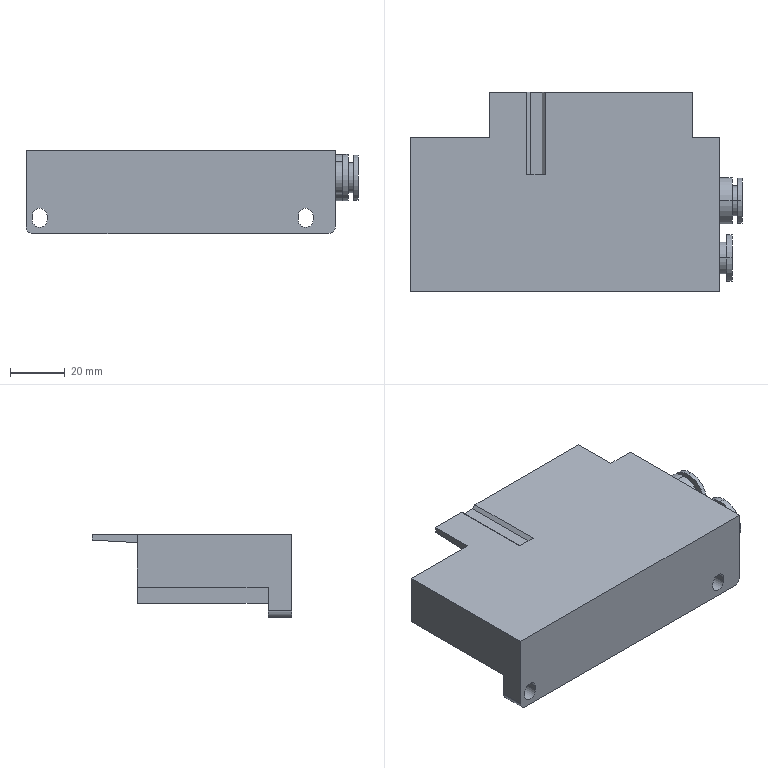Part | SolidWorks | features BaseBody 1 | 1 solid | 182 faces | box 121.7 x 73.2 x 30.5 mm | volume 162899 mm3 | plane 139 | cylinder 43 | commonest cylinder face diameters 5.5 x6 17 x4 1.085 x2 1.167 x2 1.316 x2 1.395 x2